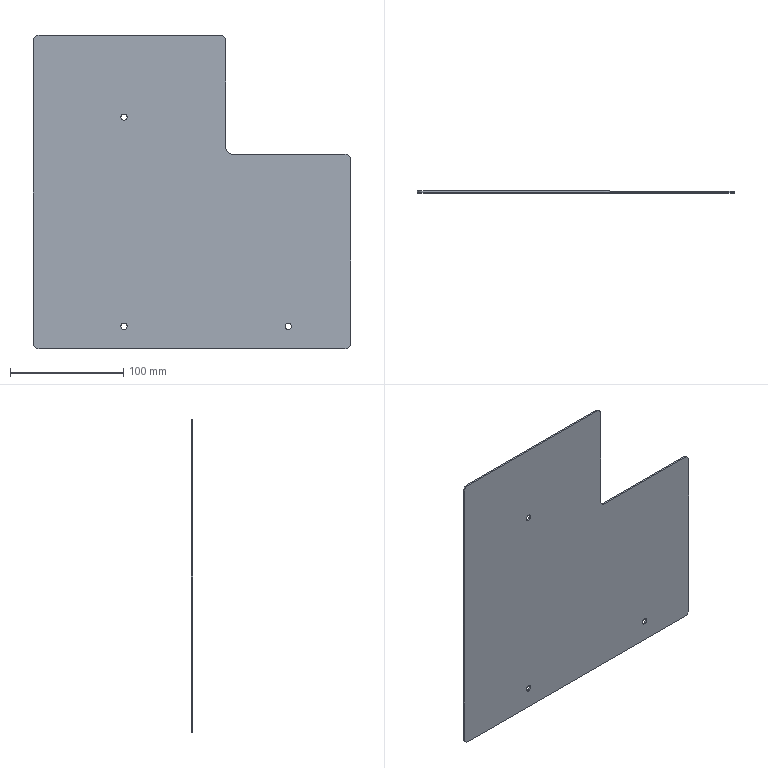Part | SolidWorks | features HoleWzd 2, Fillet 1, FlatPattern 1, ICE 1, SMBaseFlange 1, SheetMetal 1 | 1 solid | 20 faces | box 280 x 1.5 x 277 mm | volume 98876 mm3 | cylinder 12 | plane 8 | commonest cylinder face diameters 5.5 x6 10 x6
STEP:
#1=CARTESIAN_POINT('',(-60.,-1.5,63.25));
#2=VERTEX_POINT('',#1);
#3=CARTESIAN_POINT('',(-60.,-1.5,68.75));
#4=VERTEX_POINT('',#3);
#5=CARTESIAN_POINT('',(-60.,-1.5,66.));
#6=DIRECTION('',(0.,1.,0.));
#7=DIRECTION('',(0.,0.,1.));
#8=AXIS2_PLACEMENT_3D('',#5,#6,#7);
#9=CIRCLE('',#8,2.75);
#10=EDGE_CURVE('',#2,#4,#9,.T.);
#11=ORIENTED_EDGE('',*,*,#10,.F.);
#12=CARTESIAN_POINT('',(-60.,0.,63.25));
#13=VERTEX_POINT('',#12);
#14=CARTESIAN_POINT('',(-60.,0.,63.25));
#15=DIRECTION('',(0.,1.,0.));
#16=VECTOR('',#15,1000.);
#17=LINE('',#14,#16);
#18=EDGE_CURVE('',#2,#13,#17,.T.);
#19=ORIENTED_EDGE('',*,*,#18,.T.);
#20=CARTESIAN_POINT('',(-60.,0.,68.75));
#21=VERTEX_POINT('',#20);
#22=CARTESIAN_POINT('',(-60.,0.,66.));
#23=DIRECTION('',(0.,1.,0.));
#24=DIRECTION('',(0.,0.,1.));
#25=AXIS2_PLACEMENT_3D('',#22,#23,#24);
#26=CIRCLE('',#25,2.75);
#27=EDGE_CURVE('',#13,#21,#26,.T.);
#28=ORIENTED_EDGE('',*,*,#27,.T.);
#29=CARTESIAN_POINT('',(-60.,0.,68.75));
#30=DIRECTION('',(0.,1.,0.));
#31=VECTOR('',#30,1000.);
#32=LINE('',#29,#31);
#33=EDGE_CURVE('',#4,#21,#32,.T.);
#34=ORIENTED_EDGE('',*,*,#33,.F.);
#35=EDGE_LOOP('',(#11,#19,#28,#34));
#36=FACE_OUTER_BOUND('',#35,.T.);
#37=CARTESIAN_POINT('',(-60.,0.,66.));
#38=DIRECTION('',(0.,1.,0.));
#39=DIRECTION('',(0.,0.,1.));
#40=AXIS2_PLACEMENT_3D('',#37,#38,#39);
#41=CYLINDRICAL_SURFACE('',#40,2.75);
#42=ADVANCED_FACE('',(#36),#41,.F.);
#43=CARTESIAN_POINT('',(-60.,-1.5,-121.25));
#44=VERTEX_POINT('',#43);
#45=CARTESIAN_POINT('',(-60.,-1.5,-115.75));
#46=VERTEX_POINT('',#45);
#47=CARTESIAN_POINT('',(-60.,-1.5,-118.5));
#48=DIRECTION('',(0.,1.,0.));
#49=DIRECTION('',(0.,0.,1.));
#50=AXIS2_PLACEMENT_3D('',#47,#48,#49);
#51=CIRCLE('',#50,2.75);
#52=EDGE_CURVE('',#44,#46,#51,.T.);
#53=ORIENTED_EDGE('',*,*,#52,.F.);
#54=CARTESIAN_POINT('',(-60.,0.,-121.25));
#55=VERTEX_POINT('',#54);
#56=CARTESIAN_POINT('',(-60.,0.,-121.25));
#57=DIRECTION('',(0.,1.,0.));
#58=VECTOR('',#57,1000.);
#59=LINE('',#56,#58);
#60=EDGE_CURVE('',#44,#55,#59,.T.);
#61=ORIENTED_EDGE('',*,*,#60,.T.);
#62=CARTESIAN_POINT('',(-60.,0.,-115.75));
#63=VERTEX_POINT('',#62);
#64=CARTESIAN_POINT('',(-60.,0.,-118.5));
#65=DIRECTION('',(0.,1.,0.));
#66=DIRECTION('',(0.,0.,1.));
#67=AXIS2_PLACEMENT_3D('',#64,#65,#66);
#68=CIRCLE('',#67,2.75);
#69=EDGE_CURVE('',#55,#63,#68,.T.);
#70=ORIENTED_EDGE('',*,*,#69,.T.);
#71=CARTESIAN_POINT('',(-60.,0.,-115.75));
#72=DIRECTION('',(0.,1.,0.));
#73=VECTOR('',#72,1000.);
#74=LINE('',#71,#73);
#75=EDGE_CURVE('',#46,#63,#74,.T.);
#76=ORIENTED_EDGE('',*,*,#75,.F.);
#77=EDGE_LOOP('',(#53,#61,#70,#76));
#78=FACE_OUTER_BOUND('',#77,.T.);
#79=CARTESIAN_POINT('',(-60.,0.,-118.5));
#80=DIRECTION('',(0.,1.,0.));
#81=DIRECTION('',(0.,0.,1.));
#82=AXIS2_PLACEMENT_3D('',#79,#80,#81);
#83=CYLINDRICAL_SURFACE('',#82,2.75);
#84=ADVANCED_FACE('',(#78),#83,.F.);
#85=CARTESIAN_POINT('',(84.999,-1.5,-121.25));
#86=VERTEX_POINT('',#85);
#87=CARTESIAN_POINT('',(84.999,-1.5,-115.75));
#88=VERTEX_POINT('',#87);
#89=CARTESIAN_POINT('',(84.999,-1.5,-118.5));
#90=DIRECTION('',(0.,1.,0.));
#91=DIRECTION('',(0.,0.,1.));
#92=AXIS2_PLACEMENT_3D('',#89,#90,#91);
#93=CIRCLE('',#92,2.75);
#94=EDGE_CURVE('',#86,#88,#93,.T.);
#95=ORIENTED_EDGE('',*,*,#94,.F.);
#96=CARTESIAN_POINT('',(84.999,0.,-121.25));
#97=VERTEX_POINT('',#96);
#98=CARTESIAN_POINT('',(84.999,0.,-121.25));
#99=DIRECTION('',(0.,1.,0.));
#100=VECTOR('',#99,1000.);
#101=LINE('',#98,#100);
#102=EDGE_CURVE('',#86,#97,#101,.T.);
#103=ORIENTED_EDGE('',*,*,#102,.T.);
#104=CARTESIAN_POINT('',(84.999,0.,-115.75));
#105=VERTEX_POINT('',#104);
#106=CARTESIAN_POINT('',(84.999,0.,-118.5));
#107=DIRECTION('',(0.,1.,0.));
#108=DIRECTION('',(0.,0.,1.));
#109=AXIS2_PLACEMENT_3D('',#106,#107,#108);
#110=CIRCLE('',#109,2.75);
#111=EDGE_CURVE('',#97,#105,#110,.T.);
#112=ORIENTED_EDGE('',*,*,#111,.T.);
#113=CARTESIAN_POINT('',(84.999,0.,-115.75));
#114=DIRECTION('',(0.,1.,0.));
#115=VECTOR('',#114,1000.);
#116=LINE('',#113,#115);
#117=EDGE_CURVE('',#88,#105,#116,.T.);
#118=ORIENTED_EDGE('',*,*,#117,.F.);
#119=EDGE_LOOP('',(#95,#103,#112,#118));
#120=FACE_OUTER_BOUND('',#119,.T.);
#121=CARTESIAN_POINT('',(84.999,0.,-118.5));
#122=DIRECTION('',(0.,1.,0.));
#123=DIRECTION('',(0.,0.,1.));
#124=AXIS2_PLACEMENT_3D('',#121,#122,#123);
#125=CYLINDRICAL_SURFACE('',#124,2.75);
#126=ADVANCED_FACE('',(#120),#125,.F.);
#127=CARTESIAN_POINT('',(-140.,-1.5,-133.5));
#128=VERTEX_POINT('',#127);
#129=CARTESIAN_POINT('',(-140.,-1.5,133.5));
#130=VERTEX_POINT('',#129);
#131=CARTESIAN_POINT('',(-140.,-1.5,138.5));
#132=DIRECTION('',(0.,0.,1.));
#133=VECTOR('',#132,1000.);
#134=LINE('',#131,#133);
#135=EDGE_CURVE('',#128,#130,#134,.T.);
#136=ORIENTED_EDGE('',*,*,#135,.T.);
#137=CARTESIAN_POINT('',(-140.,0.,133.5));
#138=VERTEX_POINT('',#137);
#139=CARTESIAN_POINT('',(-140.,-1.5,133.5));
#140=DIRECTION('',(0.,1.,0.));
#141=VECTOR('',#140,1000.);
#142=LINE('',#139,#141);
#143=EDGE_CURVE('',#130,#138,#142,.T.);
#144=ORIENTED_EDGE('',*,*,#143,.T.);
#145=CARTESIAN_POINT('',(-140.,0.,-133.5));
#146=VERTEX_POINT('',#145);
#147=CARTESIAN_POINT('',(-140.,0.,138.5));
#148=DIRECTION('',(0.,0.,1.));
#149=VECTOR('',#148,1000.);
#150=LINE('',#147,#149);
#151=EDGE_CURVE('',#146,#138,#150,.T.);
#152=ORIENTED_EDGE('',*,*,#151,.F.);
#153=CARTESIAN_POINT('',(-140.,-1.5,-133.5));
#154=DIRECTION('',(0.,-1.,0.));
#155=VECTOR('',#154,1000.);
#156=LINE('',#153,#155);
#157=EDGE_CURVE('',#146,#128,#156,.T.);
#158=ORIENTED_EDGE('',*,*,#157,.T.);
#159=EDGE_LOOP('',(#136,#144,#152,#158));
#160=FACE_OUTER_BOUND('',#159,.T.);
#161=CARTESIAN_POINT('',(-140.,-1.5,138.5));
#162=DIRECTION('',(-1.,0.,0.));
#163=DIRECTION('',(0.,0.,1.));
#164=AXIS2_PLACEMENT_3D('',#161,#162,#163);
#165=PLANE('',#164);
#166=ADVANCED_FACE('',(#160),#165,.T.);
#167=CARTESIAN_POINT('',(135.,0.,-138.5));
#168=VERTEX_POINT('',#167);
#169=CARTESIAN_POINT('',(-135.,0.,-138.5));
#170=VERTEX_POINT('',#169);
#171=CARTESIAN_POINT('',(140.,0.,-138.5));
#172=DIRECTION('',(-1.,0.,0.));
#173=VECTOR('',#172,1000.);
#174=LINE('',#171,#173);
#175=EDGE_CURVE('',#168,#170,#174,.T.);
#176=ORIENTED_EDGE('',*,*,#175,.F.);
#177=CARTESIAN_POINT('',(135.,-1.5,-138.5));
#178=VERTEX_POINT('',#177);
#179=CARTESIAN_POINT('',(135.,-1.5,-138.5));
#180=DIRECTION('',(0.,-1.,0.));
#181=VECTOR('',#180,1000.);
#182=LINE('',#179,#181);
#183=EDGE_CURVE('',#168,#178,#182,.T.);
#184=ORIENTED_EDGE('',*,*,#183,.T.);
#185=CARTESIAN_POINT('',(-135.,-1.5,-138.5));
#186=VERTEX_POINT('',#185);
#187=CARTESIAN_POINT('',(140.,-1.5,-138.5));
#188=DIRECTION('',(-1.,0.,0.));
#189=VECTOR('',#188,1000.);
#190=LINE('',#187,#189);
#191=EDGE_CURVE('',#178,#186,#190,.T.);
#192=ORIENTED_EDGE('',*,*,#191,.T.);
#193=CARTESIAN_POINT('',(-135.,-1.5,-138.5));
#194=DIRECTION('',(0.,1.,0.));
#195=VECTOR('',#194,1000.);
#196=LINE('',#193,#195);
#197=EDGE_CURVE('',#186,#170,#196,.T.);
#198=ORIENTED_EDGE('',*,*,#197,.T.);
#199=EDGE_LOOP('',(#176,#184,#192,#198));
#200=FACE_OUTER_BOUND('',#199,.T.);
#201=CARTESIAN_POINT('',(140.,-1.5,-138.5));
#202=DIRECTION('',(0.,0.,-1.));
#203=DIRECTION('',(-1.,0.,0.));
#204=AXIS2_PLACEMENT_3D('',#201,#202,#203);
#205=PLANE('',#204);
#206=ADVANCED_FACE('',(#200),#205,.T.);
#207=CARTESIAN_POINT('',(140.,0.,28.5));
#208=VERTEX_POINT('',#207);
#209=CARTESIAN_POINT('',(140.,0.,-133.5));
#210=VERTEX_POINT('',#209);
#211=CARTESIAN_POINT('',(140.,0.,138.5));
#212=DIRECTION('',(0.,0.,-1.));
#213=VECTOR('',#212,1000.);
#214=LINE('',#211,#213);
#215=EDGE_CURVE('',#208,#210,#214,.T.);
#216=ORIENTED_EDGE('',*,*,#215,.F.);
#217=CARTESIAN_POINT('',(140.,-1.5,28.5));
#218=VERTEX_POINT('',#217);
#219=CARTESIAN_POINT('',(140.,-1.5,28.5));
#220=DIRECTION('',(0.,-1.,0.));
#221=VECTOR('',#220,1000.);
#222=LINE('',#219,#221);
#223=EDGE_CURVE('',#208,#218,#222,.T.);
#224=ORIENTED_EDGE('',*,*,#223,.T.);
#225=CARTESIAN_POINT('',(140.,-1.5,-133.5));
#226=VERTEX_POINT('',#225);
#227=CARTESIAN_POINT('',(140.,-1.5,138.5));
#228=DIRECTION('',(0.,0.,-1.));
#229=VECTOR('',#228,1000.);
#230=LINE('',#227,#229);
#231=EDGE_CURVE('',#218,#226,#230,.T.);
#232=ORIENTED_EDGE('',*,*,#231,.T.);
#233=CARTESIAN_POINT('',(140.,-1.5,-133.5));
#234=DIRECTION('',(0.,1.,0.));
#235=VECTOR('',#234,1000.);
#236=LINE('',#233,#235);
#237=EDGE_CURVE('',#226,#210,#236,.T.);
#238=ORIENTED_EDGE('',*,*,#237,.T.);
#239=EDGE_LOOP('',(#216,#224,#232,#238));
#240=FACE_OUTER_BOUND('',#239,.T.);
#241=CARTESIAN_POINT('',(140.,-1.5,138.5));
#242=DIRECTION('',(1.,0.,0.));
#243=DIRECTION('',(0.,0.,-1.));
#244=AXIS2_PLACEMENT_3D('',#241,#242,#243);
#245=PLANE('',#244);
#246=ADVANCED_FACE('',(#240),#245,.T.);
#247=CARTESIAN_POINT('',(-135.,0.,138.5));
#248=VERTEX_POINT('',#247);
#249=CARTESIAN_POINT('',(25.,0.,138.5));
#250=VERTEX_POINT('',#249);
#251=CARTESIAN_POINT('',(140.,0.,138.5));
#252=DIRECTION('',(1.,0.,0.));
#253=VECTOR('',#252,1000.);
#254=LINE('',#251,#253);
#255=EDGE_CURVE('',#248,#250,#254,.T.);
#256=ORIENTED_EDGE('',*,*,#255,.F.);
#257=CARTESIAN_POINT('',(-135.,-1.5,138.5));
#258=VERTEX_POINT('',#257);
#259=CARTESIAN_POINT('',(-135.,-1.5,138.5));
#260=DIRECTION('',(0.,-1.,0.));
#261=VECTOR('',#260,1000.);
#262=LINE('',#259,#261);
#263=EDGE_CURVE('',#248,#258,#262,.T.);
#264=ORIENTED_EDGE('',*,*,#263,.T.);
#265=CARTESIAN_POINT('',(25.,-1.5,138.5));
#266=VERTEX_POINT('',#265);
#267=CARTESIAN_POINT('',(140.,-1.5,138.5));
#268=DIRECTION('',(1.,0.,0.));
#269=VECTOR('',#268,1000.);
#270=LINE('',#267,#269);
#271=EDGE_CURVE('',#258,#266,#270,.T.);
#272=ORIENTED_EDGE('',*,*,#271,.T.);
#273=CARTESIAN_POINT('',(25.,0.,138.5));
#274=DIRECTION('',(0.,1.,0.));
#275=VECTOR('',#274,1000.);
#276=LINE('',#273,#275);
#277=EDGE_CURVE('',#266,#250,#276,.T.);
#278=ORIENTED_EDGE('',*,*,#277,.T.);
#279=EDGE_LOOP('',(#256,#264,#272,#278));
#280=FACE_OUTER_BOUND('',#279,.T.);
#281=CARTESIAN_POINT('',(140.,-1.5,138.5));
#282=DIRECTION('',(0.,0.,1.));
#283=DIRECTION('',(1.,0.,0.));
#284=AXIS2_PLACEMENT_3D('',#281,#282,#283);
#285=PLANE('',#284);
#286=ADVANCED_FACE('',(#280),#285,.T.);
#287=CARTESIAN_POINT('',(-60.,-1.5,66.));
#288=DIRECTION('',(0.,1.,0.));
#289=DIRECTION('',(0.,0.,1.));
#290=AXIS2_PLACEMENT_3D('',#287,#288,#289);
#291=CIRCLE('',#290,2.75);
#292=EDGE_CURVE('',#4,#2,#291,.T.);
#293=ORIENTED_EDGE('',*,*,#292,.T.);
#294=ORIENTED_EDGE('',*,*,#10,.T.);
#295=EDGE_LOOP('',(#293,#294));
#296=FACE_BOUND('',#295,.T.);
#297=CARTESIAN_POINT('',(-60.,-1.5,-118.5));
#298=DIRECTION('',(0.,1.,0.));
#299=DIRECTION('',(0.,0.,1.));
#300=AXIS2_PLACEMENT_3D('',#297,#298,#299);
#301=CIRCLE('',#300,2.75);
#302=EDGE_CURVE('',#46,#44,#301,.T.);
#303=ORIENTED_EDGE('',*,*,#302,.T.);
#304=ORIENTED_EDGE('',*,*,#52,.T.);
#305=EDGE_LOOP('',(#303,#304));
#306=FACE_BOUND('',#305,.T.);
#307=CARTESIAN_POINT('',(84.999,-1.5,-118.5));
#308=DIRECTION('',(0.,1.,0.));
#309=DIRECTION('',(0.,0.,1.));
#310=AXIS2_PLACEMENT_3D('',#307,#308,#309);
#311=CIRCLE('',#310,2.75);
#312=EDGE_CURVE('',#88,#86,#311,.T.);
#313=ORIENTED_EDGE('',*,*,#312,.T.);
#314=ORIENTED_EDGE('',*,*,#94,.T.);
#315=EDGE_LOOP('',(#313,#314));
#316=FACE_BOUND('',#315,.T.);
#317=ORIENTED_EDGE('',*,*,#271,.F.);
#318=CARTESIAN_POINT('',(-135.,-1.5,133.5));
#319=DIRECTION('',(0.,-1.,0.));
#320=DIRECTION('',(0.,0.,1.));
#321=AXIS2_PLACEMENT_3D('',#318,#319,#320);
#322=CIRCLE('',#321,5.);
#323=EDGE_CURVE('',#258,#130,#322,.T.);
#324=ORIENTED_EDGE('',*,*,#323,.T.);
#325=ORIENTED_EDGE('',*,*,#135,.F.);
#326=CARTESIAN_POINT('',(-135.,-1.5,-133.5));
#327=DIRECTION('',(0.,-1.,0.));
#328=DIRECTION('',(0.,0.,1.));
#329=AXIS2_PLACEMENT_3D('',#326,#327,#328);
#330=CIRCLE('',#329,5.);
#331=EDGE_CURVE('',#128,#186,#330,.T.);
#332=ORIENTED_EDGE('',*,*,#331,.T.);
#333=ORIENTED_EDGE('',*,*,#191,.F.);
#334=CARTESIAN_POINT('',(135.,-1.5,-133.5));
#335=DIRECTION('',(0.,-1.,0.));
#336=DIRECTION('',(0.,0.,1.));
#337=AXIS2_PLACEMENT_3D('',#334,#335,#336);
#338=CIRCLE('',#337,5.);
#339=EDGE_CURVE('',#178,#226,#338,.T.);
#340=ORIENTED_EDGE('',*,*,#339,.T.);
#341=ORIENTED_EDGE('',*,*,#231,.F.);
#342=CARTESIAN_POINT('',(135.,-1.5,33.5));
#343=VERTEX_POINT('',#342);
#344=CARTESIAN_POINT('',(135.,-1.5,28.5));
#345=DIRECTION('',(0.,-1.,0.));
#346=DIRECTION('',(0.,0.,1.));
#347=AXIS2_PLACEMENT_3D('',#344,#345,#346);
#348=CIRCLE('',#347,5.);
#349=EDGE_CURVE('',#218,#343,#348,.T.);
#350=ORIENTED_EDGE('',*,*,#349,.T.);
#351=CARTESIAN_POINT('',(35.,-1.5,33.5));
#352=VERTEX_POINT('',#351);
#353=CARTESIAN_POINT('',(140.,-1.5,33.5));
#354=DIRECTION('',(-1.,0.,0.));
#355=VECTOR('',#354,1000.);
#356=LINE('',#353,#355);
#357=EDGE_CURVE('',#343,#352,#356,.T.);
#358=ORIENTED_EDGE('',*,*,#357,.T.);
#359=CARTESIAN_POINT('',(30.,-1.5,38.5));
#360=VERTEX_POINT('',#359);
#361=CARTESIAN_POINT('',(35.,-1.5,38.5));
#362=DIRECTION('',(0.,1.,0.));
#363=DIRECTION('',(0.,0.,1.));
#364=AXIS2_PLACEMENT_3D('',#361,#362,#363);
#365=CIRCLE('',#364,5.);
#366=EDGE_CURVE('',#352,#360,#365,.T.);
#367=ORIENTED_EDGE('',*,*,#366,.T.);
#368=CARTESIAN_POINT('',(30.,-1.5,133.5));
#369=VERTEX_POINT('',#368);
#370=CARTESIAN_POINT('',(30.,-1.5,138.5));
#371=DIRECTION('',(0.,0.,1.));
#372=VECTOR('',#371,1000.);
#373=LINE('',#370,#372);
#374=EDGE_CURVE('',#360,#369,#373,.T.);
#375=ORIENTED_EDGE('',*,*,#374,.T.);
#376=CARTESIAN_POINT('',(25.,-1.5,133.5));
#377=DIRECTION('',(0.,-1.,0.));
#378=DIRECTION('',(0.,0.,1.));
#379=AXIS2_PLACEMENT_3D('',#376,#377,#378);
#380=CIRCLE('',#379,5.);
#381=EDGE_CURVE('',#369,#266,#380,.T.);
#382=ORIENTED_EDGE('',*,*,#381,.T.);
#383=EDGE_LOOP('',(#317,#324,#325,#332,#333,#340,#341,#350,#358,#367,#375,#382));
#384=FACE_OUTER_BOUND('',#383,.T.);
#385=CARTESIAN_POINT('',(0.,-1.5,0.));
#386=DIRECTION('',(0.,1.,0.));
#387=DIRECTION('',(0.,0.,1.));
#388=AXIS2_PLACEMENT_3D('',#385,#386,#387);
#389=PLANE('',#388);
#390=ADVANCED_FACE('',(#296,#306,#316,#384),#389,.F.);
#391=CARTESIAN_POINT('',(-60.,0.,66.));
#392=DIRECTION('',(0.,1.,0.));
#393=DIRECTION('',(0.,0.,1.));
#394=AXIS2_PLACEMENT_3D('',#391,#392,#393);
#395=CIRCLE('',#394,2.75);
#396=EDGE_CURVE('',#21,#13,#395,.T.);
#397=ORIENTED_EDGE('',*,*,#396,.F.);
#398=ORIENTED_EDGE('',*,*,#27,.F.);
#399=EDGE_LOOP('',(#397,#398));
#400=FACE_BOUND('',#399,.T.);
#401=CARTESIAN_POINT('',(-60.,0.,-118.5));
#402=DIRECTION('',(0.,1.,0.));
#403=DIRECTION('',(0.,0.,1.));
#404=AXIS2_PLACEMENT_3D('',#401,#402,#403);
#405=CIRCLE('',#404,2.75);
#406=EDGE_CURVE('',#63,#55,#405,.T.);
#407=ORIENTED_EDGE('',*,*,#406,.F.);
#408=ORIENTED_EDGE('',*,*,#69,.F.);
#409=EDGE_LOOP('',(#407,#408));
#410=FACE_BOUND('',#409,.T.);
#411=CARTESIAN_POINT('',(84.999,0.,-118.5));
#412=DIRECTION('',(0.,1.,0.));
#413=DIRECTION('',(0.,0.,1.));
#414=AXIS2_PLACEMENT_3D('',#411,#412,#413);
#415=CIRCLE('',#414,2.75);
#416=EDGE_CURVE('',#105,#97,#415,.T.);
#417=ORIENTED_EDGE('',*,*,#416,.F.);
#418=ORIENTED_EDGE('',*,*,#111,.F.);
#419=EDGE_LOOP('',(#417,#418));
#420=FACE_BOUND('',#419,.T.);
#421=ORIENTED_EDGE('',*,*,#151,.T.);
#422=CARTESIAN_POINT('',(-135.,0.,133.5));
#423=DIRECTION('',(0.,1.,0.));
#424=DIRECTION('',(0.,0.,1.));
#425=AXIS2_PLACEMENT_3D('',#422,#423,#424);
#426=CIRCLE('',#425,5.);
#427=EDGE_CURVE('',#138,#248,#426,.T.);
#428=ORIENTED_EDGE('',*,*,#427,.T.);
#429=ORIENTED_EDGE('',*,*,#255,.T.);
#430=CARTESIAN_POINT('',(30.,0.,133.5));
#431=VERTEX_POINT('',#430);
#432=CARTESIAN_POINT('',(25.,0.,133.5));
#433=DIRECTION('',(0.,1.,0.));
#434=DIRECTION('',(0.,0.,1.));
#435=AXIS2_PLACEMENT_3D('',#432,#433,#434);
#436=CIRCLE('',#435,5.);
#437=EDGE_CURVE('',#250,#431,#436,.T.);
#438=ORIENTED_EDGE('',*,*,#437,.T.);
#439=CARTESIAN_POINT('',(30.,0.,38.5));
#440=VERTEX_POINT('',#439);
#441=CARTESIAN_POINT('',(30.,0.,138.5));
#442=DIRECTION('',(0.,0.,1.));
#443=VECTOR('',#442,1000.);
#444=LINE('',#441,#443);
#445=EDGE_CURVE('',#440,#431,#444,.T.);
#446=ORIENTED_EDGE('',*,*,#445,.F.);
#447=CARTESIAN_POINT('',(35.,0.,33.5));
#448=VERTEX_POINT('',#447);
#449=CARTESIAN_POINT('',(35.,0.,38.5));
#450=DIRECTION('',(0.,-1.,0.));
#451=DIRECTION('',(0.,0.,1.));
#452=AXIS2_PLACEMENT_3D('',#449,#450,#451);
#453=CIRCLE('',#452,5.);
#454=EDGE_CURVE('',#440,#448,#453,.T.);
#455=ORIENTED_EDGE('',*,*,#454,.T.);
#456=CARTESIAN_POINT('',(135.,0.,33.5));
#457=VERTEX_POINT('',#456);
#458=CARTESIAN_POINT('',(140.,0.,33.5));
#459=DIRECTION('',(-1.,0.,0.));
#460=VECTOR('',#459,1000.);
#461=LINE('',#458,#460);
#462=EDGE_CURVE('',#457,#448,#461,.T.);
#463=ORIENTED_EDGE('',*,*,#462,.F.);
#464=CARTESIAN_POINT('',(135.,0.,28.5));
#465=DIRECTION('',(0.,1.,0.));
#466=DIRECTION('',(0.,0.,1.));
#467=AXIS2_PLACEMENT_3D('',#464,#465,#466);
#468=CIRCLE('',#467,5.);
#469=EDGE_CURVE('',#457,#208,#468,.T.);
#470=ORIENTED_EDGE('',*,*,#469,.T.);
#471=ORIENTED_EDGE('',*,*,#215,.T.);
#472=CARTESIAN_POINT('',(135.,0.,-133.5));
#473=DIRECTION('',(0.,1.,0.));
#474=DIRECTION('',(0.,0.,1.));
#475=AXIS2_PLACEMENT_3D('',#472,#473,#474);
#476=CIRCLE('',#475,5.);
#477=EDGE_CURVE('',#210,#168,#476,.T.);
#478=ORIENTED_EDGE('',*,*,#477,.T.);
#479=ORIENTED_EDGE('',*,*,#175,.T.);
#480=CARTESIAN_POINT('',(-135.,0.,-133.5));
#481=DIRECTION('',(0.,1.,0.));
#482=DIRECTION('',(0.,0.,1.));
#483=AXIS2_PLACEMENT_3D('',#480,#481,#482);
#484=CIRCLE('',#483,5.);
#485=EDGE_CURVE('',#170,#146,#484,.T.);
#486=ORIENTED_EDGE('',*,*,#485,.T.);
#487=EDGE_LOOP('',(#421,#428,#429,#438,#446,#455,#463,#470,#471,#478,#479,#486));
#488=FACE_OUTER_BOUND('',#487,.T.);
#489=CARTESIAN_POINT('',(0.,0.,0.));
#490=DIRECTION('',(0.,1.,0.));
#491=DIRECTION('',(0.,0.,1.));
#492=AXIS2_PLACEMENT_3D('',#489,#490,#491);
#493=PLANE('',#492);
#494=ADVANCED_FACE('',(#400,#410,#420,#488),#493,.T.);
#495=ORIENTED_EDGE('',*,*,#374,.F.);
#496=CARTESIAN_POINT('',(30.,0.,38.5));
#497=DIRECTION('',(0.,1.,0.));
#498=VECTOR('',#497,1000.);
#499=LINE('',#496,#498);
#500=EDGE_CURVE('',#360,#440,#499,.T.);
#501=ORIENTED_EDGE('',*,*,#500,.T.);
#502=ORIENTED_EDGE('',*,*,#445,.T.);
#503=CARTESIAN_POINT('',(30.,-1.5,133.5));
#504=DIRECTION('',(0.,-1.,0.));
#505=VECTOR('',#504,1000.);
#506=LINE('',#503,#505);
#507=EDGE_CURVE('',#431,#369,#506,.T.);
#508=ORIENTED_EDGE('',*,*,#507,.T.);
#509=EDGE_LOOP('',(#495,#501,#502,#508));
#510=FACE_OUTER_BOUND('',#509,.T.);
#511=CARTESIAN_POINT('',(30.,-1.5,138.5));
#512=DIRECTION('',(-1.,0.,0.));
#513=DIRECTION('',(0.,0.,1.));
#514=AXIS2_PLACEMENT_3D('',#511,#512,#513);
#515=PLANE('',#514);
#516=ADVANCED_FACE('',(#510),#515,.F.);
#517=ORIENTED_EDGE('',*,*,#462,.T.);
#518=CARTESIAN_POINT('',(35.,-1.5,33.5));
#519=DIRECTION('',(0.,-1.,0.));
#520=VECTOR('',#519,1000.);
#521=LINE('',#518,#520);
#522=EDGE_CURVE('',#448,#352,#521,.T.);
#523=ORIENTED_EDGE('',*,*,#522,.T.);
#524=ORIENTED_EDGE('',*,*,#357,.F.);
#525=CARTESIAN_POINT('',(135.,0.,33.5));
#526=DIRECTION('',(0.,1.,0.));
#527=VECTOR('',#526,1000.);
#528=LINE('',#525,#527);
#529=EDGE_CURVE('',#343,#457,#528,.T.);
#530=ORIENTED_EDGE('',*,*,#529,.T.);
#531=EDGE_LOOP('',(#517,#523,#524,#530));
#532=FACE_OUTER_BOUND('',#531,.T.);
#533=CARTESIAN_POINT('',(140.,-1.5,33.5));
#534=DIRECTION('',(0.,0.,-1.));
#535=DIRECTION('',(-1.,0.,0.));
#536=AXIS2_PLACEMENT_3D('',#533,#534,#535);
#537=PLANE('',#536);
#538=ADVANCED_FACE('',(#532),#537,.F.);
#539=ORIENTED_EDGE('',*,*,#366,.F.);
#540=ORIENTED_EDGE('',*,*,#522,.F.);
#541=ORIENTED_EDGE('',*,*,#454,.F.);
#542=ORIENTED_EDGE('',*,*,#500,.F.);
#543=EDGE_LOOP('',(#539,#540,#541,#542));
#544=FACE_OUTER_BOUND('',#543,.T.);
#545=CARTESIAN_POINT('',(35.,-1.5,38.5));
#546=DIRECTION('',(0.,-1.,0.));
#547=DIRECTION('',(0.,0.,-1.));
#548=AXIS2_PLACEMENT_3D('',#545,#546,#547);
#549=CYLINDRICAL_SURFACE('',#548,5.);
#550=ADVANCED_FACE('',(#544),#549,.F.);
#551=ORIENTED_EDGE('',*,*,#323,.F.);
#552=ORIENTED_EDGE('',*,*,#263,.F.);
#553=ORIENTED_EDGE('',*,*,#427,.F.);
#554=ORIENTED_EDGE('',*,*,#143,.F.);
#555=EDGE_LOOP('',(#551,#552,#553,#554));
#556=FACE_OUTER_BOUND('',#555,.T.);
#557=CARTESIAN_POINT('',(-135.,-1.5,133.5));
#558=DIRECTION('',(0.,1.,0.));
#559=DIRECTION('',(0.,0.,1.));
#560=AXIS2_PLACEMENT_3D('',#557,#558,#559);
#561=CYLINDRICAL_SURFACE('',#560,5.);
#562=ADVANCED_FACE('',(#556),#561,.T.);
#563=ORIENTED_EDGE('',*,*,#381,.F.);
#564=ORIENTED_EDGE('',*,*,#507,.F.);
#565=ORIENTED_EDGE('',*,*,#437,.F.);
#566=ORIENTED_EDGE('',*,*,#277,.F.);
#567=EDGE_LOOP('',(#563,#564,#565,#566));
#568=FACE_OUTER_BOUND('',#567,.T.);
#569=CARTESIAN_POINT('',(25.,-1.5,133.5));
#570=DIRECTION('',(0.,-1.,0.));
#571=DIRECTION('',(0.,0.,-1.));
#572=AXIS2_PLACEMENT_3D('',#569,#570,#571);
#573=CYLINDRICAL_SURFACE('',#572,5.);
#574=ADVANCED_FACE('',(#568),#573,.T.);
#575=ORIENTED_EDGE('',*,*,#349,.F.);
#576=ORIENTED_EDGE('',*,*,#223,.F.);
#577=ORIENTED_EDGE('',*,*,#469,.F.);
#578=ORIENTED_EDGE('',*,*,#529,.F.);
#579=EDGE_LOOP('',(#575,#576,#577,#578));
#580=FACE_OUTER_BOUND('',#579,.T.);
#581=CARTESIAN_POINT('',(135.,-1.5,28.5));
#582=DIRECTION('',(0.,-1.,0.));
#583=DIRECTION('',(0.,0.,-1.));
#584=AXIS2_PLACEMENT_3D('',#581,#582,#583);
#585=CYLINDRICAL_SURFACE('',#584,5.);
#586=ADVANCED_FACE('',(#580),#585,.T.);
#587=ORIENTED_EDGE('',*,*,#339,.F.);
#588=ORIENTED_EDGE('',*,*,#183,.F.);
#589=ORIENTED_EDGE('',*,*,#477,.F.);
#590=ORIENTED_EDGE('',*,*,#237,.F.);
#591=EDGE_LOOP('',(#587,#588,#589,#590));
#592=FACE_OUTER_BOUND('',#591,.T.);
#593=CARTESIAN_POINT('',(135.,-1.5,-133.5));
#594=DIRECTION('',(0.,1.,0.));
#595=DIRECTION('',(0.,0.,1.));
#596=AXIS2_PLACEMENT_3D('',#593,#594,#595);
#597=CYLINDRICAL_SURFACE('',#596,5.);
#598=ADVANCED_FACE('',(#592),#597,.T.);
#599=ORIENTED_EDGE('',*,*,#331,.F.);
#600=ORIENTED_EDGE('',*,*,#157,.F.);
#601=ORIENTED_EDGE('',*,*,#485,.F.);
#602=ORIENTED_EDGE('',*,*,#197,.F.);
#603=EDGE_LOOP('',(#599,#600,#601,#602));
#604=FACE_OUTER_BOUND('',#603,.T.);
#605=CARTESIAN_POINT('',(-135.,-1.5,-133.5));
#606=DIRECTION('',(0.,1.,0.));
#607=DIRECTION('',(0.,0.,1.));
#608=AXIS2_PLACEMENT_3D('',#605,#606,#607);
#609=CYLINDRICAL_SURFACE('',#608,5.);
#610=ADVANCED_FACE('',(#604),#609,.T.);
#611=ORIENTED_EDGE('',*,*,#102,.F.);
#612=ORIENTED_EDGE('',*,*,#312,.F.);
#613=ORIENTED_EDGE('',*,*,#117,.T.);
#614=ORIENTED_EDGE('',*,*,#416,.T.);
#615=EDGE_LOOP('',(#611,#612,#613,#614));
#616=FACE_OUTER_BOUND('',#615,.T.);
#617=CARTESIAN_POINT('',(84.999,0.,-118.5));
#618=DIRECTION('',(0.,1.,0.));
#619=DIRECTION('',(0.,0.,1.));
#620=AXIS2_PLACEMENT_3D('',#617,#618,#619);
#621=CYLINDRICAL_SURFACE('',#620,2.75);
#622=ADVANCED_FACE('',(#616),#621,.F.);
#623=ORIENTED_EDGE('',*,*,#60,.F.);
#624=ORIENTED_EDGE('',*,*,#302,.F.);
#625=ORIENTED_EDGE('',*,*,#75,.T.);
#626=ORIENTED_EDGE('',*,*,#406,.T.);
#627=EDGE_LOOP('',(#623,#624,#625,#626));
#628=FACE_OUTER_BOUND('',#627,.T.);
#629=CARTESIAN_POINT('',(-60.,0.,-118.5));
#630=DIRECTION('',(0.,1.,0.));
#631=DIRECTION('',(0.,0.,1.));
#632=AXIS2_PLACEMENT_3D('',#629,#630,#631);
#633=CYLINDRICAL_SURFACE('',#632,2.75);
#634=ADVANCED_FACE('',(#628),#633,.F.);
#635=ORIENTED_EDGE('',*,*,#18,.F.);
#636=ORIENTED_EDGE('',*,*,#292,.F.);
#637=ORIENTED_EDGE('',*,*,#33,.T.);
#638=ORIENTED_EDGE('',*,*,#396,.T.);
#639=EDGE_LOOP('',(#635,#636,#637,#638));
#640=FACE_OUTER_BOUND('',#639,.T.);
#641=CARTESIAN_POINT('',(-60.,0.,66.));
#642=DIRECTION('',(0.,1.,0.));
#643=DIRECTION('',(0.,0.,1.));
#644=AXIS2_PLACEMENT_3D('',#641,#642,#643);
#645=CYLINDRICAL_SURFACE('',#644,2.75);
#646=ADVANCED_FACE('',(#640),#645,.F.);
#647=CLOSED_SHELL('',(#42,#84,#126,#166,#206,#246,#286,#390,#494,#516,#538,#550,#562,#574,#586,#598,#610,#622,#634,#646));
#648=MANIFOLD_SOLID_BREP('',#647);
#649=CARTESIAN_POINT('',(0.,0.,0.));
#650=DIRECTION('',(0.,0.,1.));
#651=DIRECTION('',(1.,0.,0.));
#652=AXIS2_PLACEMENT_3D('',#649,#650,#651);
#653=(LENGTH_UNIT()NAMED_UNIT(*)SI_UNIT(.MILLI.,.METRE.));
#654=UNCERTAINTY_MEASURE_WITH_UNIT(LENGTH_MEASURE(0.00001),#653,'','');
#655=(NAMED_UNIT(*)PLANE_ANGLE_UNIT()SI_UNIT($,.RADIAN.));
#656=(NAMED_UNIT(*)SI_UNIT($,.STERADIAN.)SOLID_ANGLE_UNIT());
#657=(GEOMETRIC_REPRESENTATION_CONTEXT(3)GLOBAL_UNCERTAINTY_ASSIGNED_CONTEXT((#654))GLOBAL_UNIT_ASSIGNED_CONTEXT((#653,#655,#656))REPRESENTATION_CONTEXT('',''));
#658=ADVANCED_BREP_SHAPE_REPRESENTATION('',(#648,#652),#657);